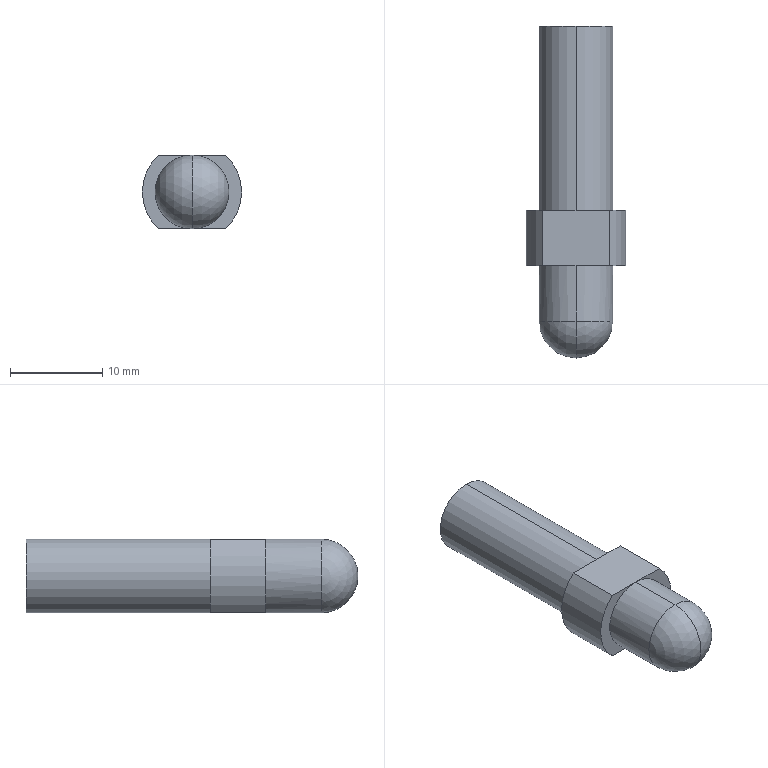Part | 1 solid | 15 faces | box 10.76 x 36 x 8 mm | volume 1905 mm3 | plane 7 | cylinder 6 | sphere 2 | commonest cylinder face diameters 8 x4 10.76 x2
STEP:
#1=CARTESIAN_POINT('',(0.,-10.,0.));
#2=VERTEX_POINT('',#1);
#3=CARTESIAN_POINT('',(0.,-6.,4.));
#4=VERTEX_POINT('',#3);
#5=CARTESIAN_POINT('',(0.,-6.,0.));
#6=DIRECTION('',(-1.,0.,0.));
#7=DIRECTION('',(0.,0.,1.));
#8=AXIS2_PLACEMENT_3D('',#5,#6,#7);
#9=CIRCLE('',#8,4.);
#10=EDGE_CURVE('',#2,#4,#9,.T.);
#11=ORIENTED_EDGE('',*,*,#10,.F.);
#12=CARTESIAN_POINT('',(0.,-6.,-4.));
#13=VERTEX_POINT('',#12);
#14=CARTESIAN_POINT('',(0.,-6.,0.));
#15=DIRECTION('',(1.,0.,0.));
#16=DIRECTION('',(0.,0.,-1.));
#17=AXIS2_PLACEMENT_3D('',#14,#15,#16);
#18=CIRCLE('',#17,4.);
#19=EDGE_CURVE('',#2,#13,#18,.T.);
#20=ORIENTED_EDGE('',*,*,#19,.T.);
#21=CARTESIAN_POINT('',(0.,-6.,0.));
#22=DIRECTION('',(0.,-1.,0.));
#23=DIRECTION('',(0.,0.,-1.));
#24=AXIS2_PLACEMENT_3D('',#21,#22,#23);
#25=CIRCLE('',#24,4.);
#26=EDGE_CURVE('',#13,#4,#25,.T.);
#27=ORIENTED_EDGE('',*,*,#26,.T.);
#28=EDGE_LOOP('',(#11,#20,#27));
#29=FACE_OUTER_BOUND('',#28,.T.);
#30=CARTESIAN_POINT('',(0.,-6.,0.));
#31=DIRECTION('',(1.,0.,0.));
#32=DIRECTION('',(0.,0.,1.));
#33=AXIS2_PLACEMENT_3D('',#30,#31,#32);
#34=SPHERICAL_SURFACE('',#33,4.);
#35=ADVANCED_FACE('',(#29),#34,.T.);
#36=ORIENTED_EDGE('',*,*,#26,.F.);
#37=CARTESIAN_POINT('',(0.,0.,-4.));
#38=VERTEX_POINT('',#37);
#39=CARTESIAN_POINT('',(0.,-6.,-4.));
#40=DIRECTION('',(0.,1.,0.));
#41=VECTOR('',#40,1000.);
#42=LINE('',#39,#41);
#43=EDGE_CURVE('',#13,#38,#42,.T.);
#44=ORIENTED_EDGE('',*,*,#43,.T.);
#45=CARTESIAN_POINT('',(0.,0.,4.));
#46=VERTEX_POINT('',#45);
#47=CARTESIAN_POINT('',(0.,0.,0.));
#48=DIRECTION('',(0.,-1.,0.));
#49=DIRECTION('',(0.,0.,-1.));
#50=AXIS2_PLACEMENT_3D('',#47,#48,#49);
#51=CIRCLE('',#50,4.);
#52=EDGE_CURVE('',#38,#46,#51,.T.);
#53=ORIENTED_EDGE('',*,*,#52,.T.);
#54=CARTESIAN_POINT('',(0.,-6.,4.));
#55=DIRECTION('',(0.,1.,0.));
#56=VECTOR('',#55,1000.);
#57=LINE('',#54,#56);
#58=EDGE_CURVE('',#4,#46,#57,.T.);
#59=ORIENTED_EDGE('',*,*,#58,.F.);
#60=EDGE_LOOP('',(#36,#44,#53,#59));
#61=FACE_OUTER_BOUND('',#60,.T.);
#62=CARTESIAN_POINT('',(0.,-6.,0.));
#63=DIRECTION('',(0.,1.,0.));
#64=DIRECTION('',(0.,0.,1.));
#65=AXIS2_PLACEMENT_3D('',#62,#63,#64);
#66=CYLINDRICAL_SURFACE('',#65,4.);
#67=ADVANCED_FACE('',(#61),#66,.T.);
#68=CARTESIAN_POINT('',(0.,26.,4.));
#69=VERTEX_POINT('',#68);
#70=CARTESIAN_POINT('',(0.,26.,-4.));
#71=VERTEX_POINT('',#70);
#72=CARTESIAN_POINT('',(0.,26.,0.));
#73=DIRECTION('',(0.,1.,0.));
#74=DIRECTION('',(0.,0.,1.));
#75=AXIS2_PLACEMENT_3D('',#72,#73,#74);
#76=CIRCLE('',#75,4.);
#77=EDGE_CURVE('',#69,#71,#76,.T.);
#78=ORIENTED_EDGE('',*,*,#77,.F.);
#79=CARTESIAN_POINT('',(0.,6.,4.));
#80=VERTEX_POINT('',#79);
#81=CARTESIAN_POINT('',(0.,26.,4.));
#82=DIRECTION('',(0.,-1.,0.));
#83=VECTOR('',#82,1000.);
#84=LINE('',#81,#83);
#85=EDGE_CURVE('',#69,#80,#84,.T.);
#86=ORIENTED_EDGE('',*,*,#85,.T.);
#87=CARTESIAN_POINT('',(0.,6.,-4.));
#88=VERTEX_POINT('',#87);
#89=CARTESIAN_POINT('',(0.,6.,0.));
#90=DIRECTION('',(0.,1.,0.));
#91=DIRECTION('',(0.,0.,1.));
#92=AXIS2_PLACEMENT_3D('',#89,#90,#91);
#93=CIRCLE('',#92,4.);
#94=EDGE_CURVE('',#80,#88,#93,.T.);
#95=ORIENTED_EDGE('',*,*,#94,.T.);
#96=CARTESIAN_POINT('',(0.,26.,-4.));
#97=DIRECTION('',(0.,-1.,0.));
#98=VECTOR('',#97,1000.);
#99=LINE('',#96,#98);
#100=EDGE_CURVE('',#71,#88,#99,.T.);
#101=ORIENTED_EDGE('',*,*,#100,.F.);
#102=EDGE_LOOP('',(#78,#86,#95,#101));
#103=FACE_OUTER_BOUND('',#102,.T.);
#104=CARTESIAN_POINT('',(0.,26.,0.));
#105=DIRECTION('',(0.,-1.,0.));
#106=DIRECTION('',(0.,0.,-1.));
#107=AXIS2_PLACEMENT_3D('',#104,#105,#106);
#108=CYLINDRICAL_SURFACE('',#107,4.);
#109=ADVANCED_FACE('',(#103),#108,.T.);
#110=ORIENTED_EDGE('',*,*,#52,.F.);
#111=CARTESIAN_POINT('',(3.598,0.,-4.));
#112=VERTEX_POINT('',#111);
#113=CARTESIAN_POINT('',(0.,0.,-4.));
#114=DIRECTION('',(1.,0.,0.));
#115=VECTOR('',#114,1000.);
#116=LINE('',#113,#115);
#117=EDGE_CURVE('',#38,#112,#116,.T.);
#118=ORIENTED_EDGE('',*,*,#117,.T.);
#119=CARTESIAN_POINT('',(3.598,0.,4.));
#120=VERTEX_POINT('',#119);
#121=CARTESIAN_POINT('',(0.,0.,0.));
#122=DIRECTION('',(0.,1.,0.));
#123=DIRECTION('',(0.,0.,1.));
#124=AXIS2_PLACEMENT_3D('',#121,#122,#123);
#125=CIRCLE('',#124,5.38);
#126=EDGE_CURVE('',#120,#112,#125,.T.);
#127=ORIENTED_EDGE('',*,*,#126,.F.);
#128=CARTESIAN_POINT('',(0.,0.,4.));
#129=DIRECTION('',(-1.,0.,0.));
#130=VECTOR('',#129,1000.);
#131=LINE('',#128,#130);
#132=EDGE_CURVE('',#120,#46,#131,.T.);
#133=ORIENTED_EDGE('',*,*,#132,.T.);
#134=EDGE_LOOP('',(#110,#118,#127,#133));
#135=FACE_OUTER_BOUND('',#134,.T.);
#136=CARTESIAN_POINT('',(0.,0.,0.));
#137=DIRECTION('',(0.,1.,0.));
#138=DIRECTION('',(1.,0.,0.));
#139=AXIS2_PLACEMENT_3D('',#136,#137,#138);
#140=PLANE('',#139);
#141=ADVANCED_FACE('',(#135),#140,.F.);
#142=ORIENTED_EDGE('',*,*,#94,.F.);
#143=CARTESIAN_POINT('',(3.598,6.,4.));
#144=VERTEX_POINT('',#143);
#145=CARTESIAN_POINT('',(-6.5,6.,4.));
#146=DIRECTION('',(1.,0.,0.));
#147=VECTOR('',#146,1000.);
#148=LINE('',#145,#147);
#149=EDGE_CURVE('',#80,#144,#148,.T.);
#150=ORIENTED_EDGE('',*,*,#149,.T.);
#151=CARTESIAN_POINT('',(3.598,6.,-4.));
#152=VERTEX_POINT('',#151);
#153=CARTESIAN_POINT('',(0.,6.,0.));
#154=DIRECTION('',(0.,1.,0.));
#155=DIRECTION('',(0.,0.,1.));
#156=AXIS2_PLACEMENT_3D('',#153,#154,#155);
#157=CIRCLE('',#156,5.38);
#158=EDGE_CURVE('',#144,#152,#157,.T.);
#159=ORIENTED_EDGE('',*,*,#158,.T.);
#160=CARTESIAN_POINT('',(-6.5,6.,-4.));
#161=DIRECTION('',(-1.,0.,0.));
#162=VECTOR('',#161,1000.);
#163=LINE('',#160,#162);
#164=EDGE_CURVE('',#152,#88,#163,.T.);
#165=ORIENTED_EDGE('',*,*,#164,.T.);
#166=EDGE_LOOP('',(#142,#150,#159,#165));
#167=FACE_OUTER_BOUND('',#166,.T.);
#168=CARTESIAN_POINT('',(0.,6.,0.));
#169=DIRECTION('',(0.,1.,0.));
#170=DIRECTION('',(1.,0.,0.));
#171=AXIS2_PLACEMENT_3D('',#168,#169,#170);
#172=PLANE('',#171);
#173=ADVANCED_FACE('',(#167),#172,.T.);
#174=CARTESIAN_POINT('',(-3.598,6.,-4.));
#175=VERTEX_POINT('',#174);
#176=CARTESIAN_POINT('',(-3.598,6.,4.));
#177=VERTEX_POINT('',#176);
#178=CARTESIAN_POINT('',(0.,6.,0.));
#179=DIRECTION('',(0.,1.,0.));
#180=DIRECTION('',(0.,0.,1.));
#181=AXIS2_PLACEMENT_3D('',#178,#179,#180);
#182=CIRCLE('',#181,5.38);
#183=EDGE_CURVE('',#175,#177,#182,.T.);
#184=ORIENTED_EDGE('',*,*,#183,.F.);
#185=CARTESIAN_POINT('',(-3.598,0.,-4.));
#186=VERTEX_POINT('',#185);
#187=CARTESIAN_POINT('',(-3.598,6.,-4.));
#188=DIRECTION('',(0.,-1.,0.));
#189=VECTOR('',#188,1000.);
#190=LINE('',#187,#189);
#191=EDGE_CURVE('',#175,#186,#190,.T.);
#192=ORIENTED_EDGE('',*,*,#191,.T.);
#193=CARTESIAN_POINT('',(-3.598,0.,4.));
#194=VERTEX_POINT('',#193);
#195=CARTESIAN_POINT('',(0.,0.,0.));
#196=DIRECTION('',(0.,1.,0.));
#197=DIRECTION('',(0.,0.,1.));
#198=AXIS2_PLACEMENT_3D('',#195,#196,#197);
#199=CIRCLE('',#198,5.38);
#200=EDGE_CURVE('',#186,#194,#199,.T.);
#201=ORIENTED_EDGE('',*,*,#200,.T.);
#202=CARTESIAN_POINT('',(-3.598,6.,4.));
#203=DIRECTION('',(0.,1.,0.));
#204=VECTOR('',#203,1000.);
#205=LINE('',#202,#204);
#206=EDGE_CURVE('',#194,#177,#205,.T.);
#207=ORIENTED_EDGE('',*,*,#206,.T.);
#208=EDGE_LOOP('',(#184,#192,#201,#207));
#209=FACE_OUTER_BOUND('',#208,.T.);
#210=CARTESIAN_POINT('',(0.,6.,0.));
#211=DIRECTION('',(0.,-1.,0.));
#212=DIRECTION('',(0.,0.,-1.));
#213=AXIS2_PLACEMENT_3D('',#210,#211,#212);
#214=CYLINDRICAL_SURFACE('',#213,5.38);
#215=ADVANCED_FACE('',(#209),#214,.T.);
#216=ORIENTED_EDGE('',*,*,#126,.T.);
#217=CARTESIAN_POINT('',(3.598,6.,-4.));
#218=DIRECTION('',(0.,1.,0.));
#219=VECTOR('',#218,1000.);
#220=LINE('',#217,#219);
#221=EDGE_CURVE('',#112,#152,#220,.T.);
#222=ORIENTED_EDGE('',*,*,#221,.T.);
#223=ORIENTED_EDGE('',*,*,#158,.F.);
#224=CARTESIAN_POINT('',(3.598,6.,4.));
#225=DIRECTION('',(0.,-1.,0.));
#226=VECTOR('',#225,1000.);
#227=LINE('',#224,#226);
#228=EDGE_CURVE('',#144,#120,#227,.T.);
#229=ORIENTED_EDGE('',*,*,#228,.T.);
#230=EDGE_LOOP('',(#216,#222,#223,#229));
#231=FACE_OUTER_BOUND('',#230,.T.);
#232=CARTESIAN_POINT('',(0.,6.,0.));
#233=DIRECTION('',(0.,-1.,0.));
#234=DIRECTION('',(0.,0.,-1.));
#235=AXIS2_PLACEMENT_3D('',#232,#233,#234);
#236=CYLINDRICAL_SURFACE('',#235,5.38);
#237=ADVANCED_FACE('',(#231),#236,.T.);
#238=CARTESIAN_POINT('',(0.,6.,0.));
#239=DIRECTION('',(0.,1.,0.));
#240=DIRECTION('',(0.,0.,1.));
#241=AXIS2_PLACEMENT_3D('',#238,#239,#240);
#242=CIRCLE('',#241,4.);
#243=EDGE_CURVE('',#88,#80,#242,.T.);
#244=ORIENTED_EDGE('',*,*,#243,.F.);
#245=CARTESIAN_POINT('',(-6.5,6.,-4.));
#246=DIRECTION('',(-1.,0.,0.));
#247=VECTOR('',#246,1000.);
#248=LINE('',#245,#247);
#249=EDGE_CURVE('',#88,#175,#248,.T.);
#250=ORIENTED_EDGE('',*,*,#249,.T.);
#251=ORIENTED_EDGE('',*,*,#183,.T.);
#252=CARTESIAN_POINT('',(-6.5,6.,4.));
#253=DIRECTION('',(1.,0.,0.));
#254=VECTOR('',#253,1000.);
#255=LINE('',#252,#254);
#256=EDGE_CURVE('',#177,#80,#255,.T.);
#257=ORIENTED_EDGE('',*,*,#256,.T.);
#258=EDGE_LOOP('',(#244,#250,#251,#257));
#259=FACE_OUTER_BOUND('',#258,.T.);
#260=CARTESIAN_POINT('',(0.,6.,0.));
#261=DIRECTION('',(0.,1.,0.));
#262=DIRECTION('',(1.,0.,0.));
#263=AXIS2_PLACEMENT_3D('',#260,#261,#262);
#264=PLANE('',#263);
#265=ADVANCED_FACE('',(#259),#264,.T.);
#266=CARTESIAN_POINT('',(0.,0.,0.));
#267=DIRECTION('',(0.,-1.,0.));
#268=DIRECTION('',(0.,0.,-1.));
#269=AXIS2_PLACEMENT_3D('',#266,#267,#268);
#270=CIRCLE('',#269,4.);
#271=EDGE_CURVE('',#46,#38,#270,.T.);
#272=ORIENTED_EDGE('',*,*,#271,.F.);
#273=CARTESIAN_POINT('',(0.,0.,4.));
#274=DIRECTION('',(-1.,0.,0.));
#275=VECTOR('',#274,1000.);
#276=LINE('',#273,#275);
#277=EDGE_CURVE('',#46,#194,#276,.T.);
#278=ORIENTED_EDGE('',*,*,#277,.T.);
#279=ORIENTED_EDGE('',*,*,#200,.F.);
#280=CARTESIAN_POINT('',(0.,0.,-4.));
#281=DIRECTION('',(1.,0.,0.));
#282=VECTOR('',#281,1000.);
#283=LINE('',#280,#282);
#284=EDGE_CURVE('',#186,#38,#283,.T.);
#285=ORIENTED_EDGE('',*,*,#284,.T.);
#286=EDGE_LOOP('',(#272,#278,#279,#285));
#287=FACE_OUTER_BOUND('',#286,.T.);
#288=CARTESIAN_POINT('',(0.,0.,0.));
#289=DIRECTION('',(0.,1.,0.));
#290=DIRECTION('',(1.,0.,0.));
#291=AXIS2_PLACEMENT_3D('',#288,#289,#290);
#292=PLANE('',#291);
#293=ADVANCED_FACE('',(#287),#292,.F.);
#294=ORIENTED_EDGE('',*,*,#256,.F.);
#295=ORIENTED_EDGE('',*,*,#206,.F.);
#296=ORIENTED_EDGE('',*,*,#277,.F.);
#297=ORIENTED_EDGE('',*,*,#132,.F.);
#298=ORIENTED_EDGE('',*,*,#228,.F.);
#299=ORIENTED_EDGE('',*,*,#149,.F.);
#300=EDGE_LOOP('',(#294,#295,#296,#297,#298,#299));
#301=FACE_OUTER_BOUND('',#300,.T.);
#302=CARTESIAN_POINT('',(-6.5,6.,4.));
#303=DIRECTION('',(0.,0.,-1.));
#304=DIRECTION('',(0.,-1.,0.));
#305=AXIS2_PLACEMENT_3D('',#302,#303,#304);
#306=PLANE('',#305);
#307=ADVANCED_FACE('',(#301),#306,.F.);
#308=ORIENTED_EDGE('',*,*,#164,.F.);
#309=ORIENTED_EDGE('',*,*,#221,.F.);
#310=ORIENTED_EDGE('',*,*,#117,.F.);
#311=ORIENTED_EDGE('',*,*,#284,.F.);
#312=ORIENTED_EDGE('',*,*,#191,.F.);
#313=ORIENTED_EDGE('',*,*,#249,.F.);
#314=EDGE_LOOP('',(#308,#309,#310,#311,#312,#313));
#315=FACE_OUTER_BOUND('',#314,.T.);
#316=CARTESIAN_POINT('',(-6.5,6.,-4.));
#317=DIRECTION('',(0.,0.,1.));
#318=DIRECTION('',(1.,0.,0.));
#319=AXIS2_PLACEMENT_3D('',#316,#317,#318);
#320=PLANE('',#319);
#321=ADVANCED_FACE('',(#315),#320,.F.);
#322=ORIENTED_EDGE('',*,*,#85,.F.);
#323=CARTESIAN_POINT('',(0.,26.,0.));
#324=DIRECTION('',(0.,1.,0.));
#325=DIRECTION('',(0.,0.,1.));
#326=AXIS2_PLACEMENT_3D('',#323,#324,#325);
#327=CIRCLE('',#326,4.);
#328=EDGE_CURVE('',#71,#69,#327,.T.);
#329=ORIENTED_EDGE('',*,*,#328,.F.);
#330=ORIENTED_EDGE('',*,*,#100,.T.);
#331=ORIENTED_EDGE('',*,*,#243,.T.);
#332=EDGE_LOOP('',(#322,#329,#330,#331));
#333=FACE_OUTER_BOUND('',#332,.T.);
#334=CARTESIAN_POINT('',(0.,26.,0.));
#335=DIRECTION('',(0.,-1.,0.));
#336=DIRECTION('',(0.,0.,-1.));
#337=AXIS2_PLACEMENT_3D('',#334,#335,#336);
#338=CYLINDRICAL_SURFACE('',#337,4.);
#339=ADVANCED_FACE('',(#333),#338,.T.);
#340=ORIENTED_EDGE('',*,*,#328,.T.);
#341=ORIENTED_EDGE('',*,*,#77,.T.);
#342=EDGE_LOOP('',(#340,#341));
#343=FACE_OUTER_BOUND('',#342,.T.);
#344=CARTESIAN_POINT('',(0.,26.,0.));
#345=DIRECTION('',(0.,1.,0.));
#346=DIRECTION('',(1.,0.,0.));
#347=AXIS2_PLACEMENT_3D('',#344,#345,#346);
#348=PLANE('',#347);
#349=ADVANCED_FACE('',(#343),#348,.T.);
#350=ORIENTED_EDGE('',*,*,#43,.F.);
#351=CARTESIAN_POINT('',(0.,-6.,0.));
#352=DIRECTION('',(0.,-1.,0.));
#353=DIRECTION('',(0.,0.,-1.));
#354=AXIS2_PLACEMENT_3D('',#351,#352,#353);
#355=CIRCLE('',#354,4.);
#356=EDGE_CURVE('',#4,#13,#355,.T.);
#357=ORIENTED_EDGE('',*,*,#356,.F.);
#358=ORIENTED_EDGE('',*,*,#58,.T.);
#359=ORIENTED_EDGE('',*,*,#271,.T.);
#360=EDGE_LOOP('',(#350,#357,#358,#359));
#361=FACE_OUTER_BOUND('',#360,.T.);
#362=CARTESIAN_POINT('',(0.,-6.,0.));
#363=DIRECTION('',(0.,1.,0.));
#364=DIRECTION('',(0.,0.,1.));
#365=AXIS2_PLACEMENT_3D('',#362,#363,#364);
#366=CYLINDRICAL_SURFACE('',#365,4.);
#367=ADVANCED_FACE('',(#361),#366,.T.);
#368=ORIENTED_EDGE('',*,*,#19,.F.);
#369=ORIENTED_EDGE('',*,*,#10,.T.);
#370=ORIENTED_EDGE('',*,*,#356,.T.);
#371=EDGE_LOOP('',(#368,#369,#370));
#372=FACE_OUTER_BOUND('',#371,.T.);
#373=CARTESIAN_POINT('',(0.,-6.,0.));
#374=DIRECTION('',(1.,0.,0.));
#375=DIRECTION('',(0.,0.,1.));
#376=AXIS2_PLACEMENT_3D('',#373,#374,#375);
#377=SPHERICAL_SURFACE('',#376,4.);
#378=ADVANCED_FACE('',(#372),#377,.T.);
#379=CLOSED_SHELL('',(#35,#67,#109,#141,#173,#215,#237,#265,#293,#307,#321,#339,#349,#367,#378));
#380=MANIFOLD_SOLID_BREP('',#379);
#381=CARTESIAN_POINT('',(0.,0.,0.));
#382=DIRECTION('',(0.,0.,1.));
#383=DIRECTION('',(1.,0.,0.));
#384=AXIS2_PLACEMENT_3D('',#381,#382,#383);
#385=(LENGTH_UNIT()NAMED_UNIT(*)SI_UNIT(.MILLI.,.METRE.));
#386=UNCERTAINTY_MEASURE_WITH_UNIT(LENGTH_MEASURE(0.00001),#385,'','');
#387=(NAMED_UNIT(*)PLANE_ANGLE_UNIT()SI_UNIT($,.RADIAN.));
#388=(NAMED_UNIT(*)SI_UNIT($,.STERADIAN.)SOLID_ANGLE_UNIT());
#389=(GEOMETRIC_REPRESENTATION_CONTEXT(3)GLOBAL_UNCERTAINTY_ASSIGNED_CONTEXT((#386))GLOBAL_UNIT_ASSIGNED_CONTEXT((#385,#387,#388))REPRESENTATION_CONTEXT('',''));
#390=ADVANCED_BREP_SHAPE_REPRESENTATION('',(#380,#384),#389);